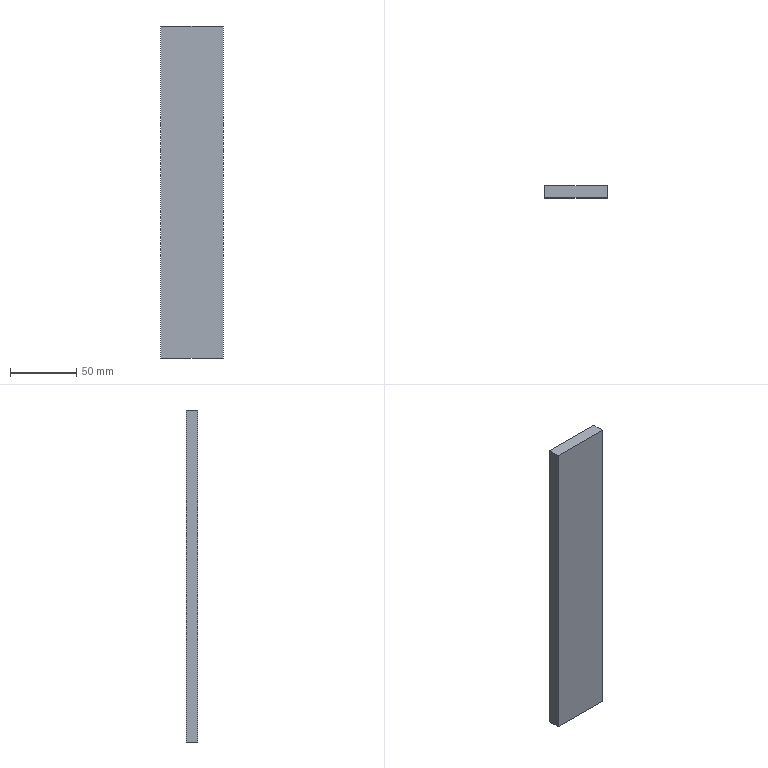Part | STEP file | Squeegee rubber | 1 solid | 6 faces | box 47 x 9 x 250 mm | volume 105750 mm3 | plane 6
STEP:
#1=CARTESIAN_POINT('',(29.,4.5,-250.));
#2=VERTEX_POINT('',#1);
#3=CARTESIAN_POINT('',(29.,-4.5,-250.));
#4=VERTEX_POINT('',#3);
#5=CARTESIAN_POINT('',(29.,4.5,-250.));
#6=DIRECTION('',(0.,-1.,0.));
#7=VECTOR('',#6,1000.);
#8=LINE('',#5,#7);
#9=EDGE_CURVE('',#2,#4,#8,.T.);
#10=ORIENTED_EDGE('',*,*,#9,.F.);
#11=CARTESIAN_POINT('',(76.,4.5,-250.));
#12=VERTEX_POINT('',#11);
#13=CARTESIAN_POINT('',(29.,4.5,-250.));
#14=DIRECTION('',(-1.,0.,0.));
#15=VECTOR('',#14,1000.);
#16=LINE('',#13,#15);
#17=EDGE_CURVE('',#12,#2,#16,.T.);
#18=ORIENTED_EDGE('',*,*,#17,.F.);
#19=CARTESIAN_POINT('',(76.,-4.5,-250.));
#20=VERTEX_POINT('',#19);
#21=CARTESIAN_POINT('',(76.,4.5,-250.));
#22=DIRECTION('',(0.,1.,0.));
#23=VECTOR('',#22,1000.);
#24=LINE('',#21,#23);
#25=EDGE_CURVE('',#20,#12,#24,.T.);
#26=ORIENTED_EDGE('',*,*,#25,.F.);
#27=CARTESIAN_POINT('',(29.,-4.5,-250.));
#28=DIRECTION('',(1.,0.,0.));
#29=VECTOR('',#28,1000.);
#30=LINE('',#27,#29);
#31=EDGE_CURVE('',#4,#20,#30,.T.);
#32=ORIENTED_EDGE('',*,*,#31,.F.);
#33=EDGE_LOOP('',(#10,#18,#26,#32));
#34=FACE_OUTER_BOUND('',#33,.T.);
#35=CARTESIAN_POINT('',(0.,0.,-250.));
#36=DIRECTION('',(0.,0.,-1.));
#37=DIRECTION('',(-1.,0.,0.));
#38=AXIS2_PLACEMENT_3D('',#35,#36,#37);
#39=PLANE('',#38);
#40=ADVANCED_FACE('',(#34),#39,.T.);
#41=CARTESIAN_POINT('',(29.,4.5,0.));
#42=VERTEX_POINT('',#41);
#43=CARTESIAN_POINT('',(29.,-4.5,0.));
#44=VERTEX_POINT('',#43);
#45=CARTESIAN_POINT('',(29.,4.5,0.));
#46=DIRECTION('',(0.,-1.,0.));
#47=VECTOR('',#46,1000.);
#48=LINE('',#45,#47);
#49=EDGE_CURVE('',#42,#44,#48,.T.);
#50=ORIENTED_EDGE('',*,*,#49,.T.);
#51=CARTESIAN_POINT('',(76.,-4.5,0.));
#52=VERTEX_POINT('',#51);
#53=CARTESIAN_POINT('',(29.,-4.5,0.));
#54=DIRECTION('',(1.,0.,0.));
#55=VECTOR('',#54,1000.);
#56=LINE('',#53,#55);
#57=EDGE_CURVE('',#44,#52,#56,.T.);
#58=ORIENTED_EDGE('',*,*,#57,.T.);
#59=CARTESIAN_POINT('',(76.,4.5,0.));
#60=VERTEX_POINT('',#59);
#61=CARTESIAN_POINT('',(76.,4.5,0.));
#62=DIRECTION('',(0.,1.,0.));
#63=VECTOR('',#62,1000.);
#64=LINE('',#61,#63);
#65=EDGE_CURVE('',#52,#60,#64,.T.);
#66=ORIENTED_EDGE('',*,*,#65,.T.);
#67=CARTESIAN_POINT('',(29.,4.5,0.));
#68=DIRECTION('',(-1.,0.,0.));
#69=VECTOR('',#68,1000.);
#70=LINE('',#67,#69);
#71=EDGE_CURVE('',#60,#42,#70,.T.);
#72=ORIENTED_EDGE('',*,*,#71,.T.);
#73=EDGE_LOOP('',(#50,#58,#66,#72));
#74=FACE_OUTER_BOUND('',#73,.T.);
#75=CARTESIAN_POINT('',(0.,0.,0.));
#76=DIRECTION('',(0.,0.,1.));
#77=DIRECTION('',(1.,0.,0.));
#78=AXIS2_PLACEMENT_3D('',#75,#76,#77);
#79=PLANE('',#78);
#80=ADVANCED_FACE('',(#74),#79,.T.);
#81=CARTESIAN_POINT('',(29.,-4.5,-297.854));
#82=DIRECTION('',(0.,0.,1.));
#83=VECTOR('',#82,1000.);
#84=LINE('',#81,#83);
#85=EDGE_CURVE('',#4,#44,#84,.T.);
#86=ORIENTED_EDGE('',*,*,#85,.F.);
#87=ORIENTED_EDGE('',*,*,#31,.T.);
#88=CARTESIAN_POINT('',(76.,-4.5,-297.854));
#89=DIRECTION('',(0.,0.,1.));
#90=VECTOR('',#89,1000.);
#91=LINE('',#88,#90);
#92=EDGE_CURVE('',#20,#52,#91,.T.);
#93=ORIENTED_EDGE('',*,*,#92,.T.);
#94=ORIENTED_EDGE('',*,*,#57,.F.);
#95=EDGE_LOOP('',(#86,#87,#93,#94));
#96=FACE_OUTER_BOUND('',#95,.T.);
#97=CARTESIAN_POINT('',(29.,-4.5,-297.854));
#98=DIRECTION('',(0.,-1.,0.));
#99=DIRECTION('',(0.,0.,-1.));
#100=AXIS2_PLACEMENT_3D('',#97,#98,#99);
#101=PLANE('',#100);
#102=ADVANCED_FACE('',(#96),#101,.T.);
#103=ORIENTED_EDGE('',*,*,#92,.F.);
#104=ORIENTED_EDGE('',*,*,#25,.T.);
#105=CARTESIAN_POINT('',(76.,4.5,-297.854));
#106=DIRECTION('',(0.,0.,1.));
#107=VECTOR('',#106,1000.);
#108=LINE('',#105,#107);
#109=EDGE_CURVE('',#12,#60,#108,.T.);
#110=ORIENTED_EDGE('',*,*,#109,.T.);
#111=ORIENTED_EDGE('',*,*,#65,.F.);
#112=EDGE_LOOP('',(#103,#104,#110,#111));
#113=FACE_OUTER_BOUND('',#112,.T.);
#114=CARTESIAN_POINT('',(76.,4.5,-297.854));
#115=DIRECTION('',(1.,0.,0.));
#116=DIRECTION('',(0.,0.,-1.));
#117=AXIS2_PLACEMENT_3D('',#114,#115,#116);
#118=PLANE('',#117);
#119=ADVANCED_FACE('',(#113),#118,.T.);
#120=ORIENTED_EDGE('',*,*,#109,.F.);
#121=ORIENTED_EDGE('',*,*,#17,.T.);
#122=CARTESIAN_POINT('',(29.,4.5,-297.854));
#123=DIRECTION('',(0.,0.,1.));
#124=VECTOR('',#123,1000.);
#125=LINE('',#122,#124);
#126=EDGE_CURVE('',#2,#42,#125,.T.);
#127=ORIENTED_EDGE('',*,*,#126,.T.);
#128=ORIENTED_EDGE('',*,*,#71,.F.);
#129=EDGE_LOOP('',(#120,#121,#127,#128));
#130=FACE_OUTER_BOUND('',#129,.T.);
#131=CARTESIAN_POINT('',(29.,4.5,-297.854));
#132=DIRECTION('',(0.,1.,0.));
#133=DIRECTION('',(0.,0.,1.));
#134=AXIS2_PLACEMENT_3D('',#131,#132,#133);
#135=PLANE('',#134);
#136=ADVANCED_FACE('',(#130),#135,.T.);
#137=ORIENTED_EDGE('',*,*,#126,.F.);
#138=ORIENTED_EDGE('',*,*,#9,.T.);
#139=ORIENTED_EDGE('',*,*,#85,.T.);
#140=ORIENTED_EDGE('',*,*,#49,.F.);
#141=EDGE_LOOP('',(#137,#138,#139,#140));
#142=FACE_OUTER_BOUND('',#141,.T.);
#143=CARTESIAN_POINT('',(29.,4.5,-297.854));
#144=DIRECTION('',(-1.,0.,0.));
#145=DIRECTION('',(0.,0.,1.));
#146=AXIS2_PLACEMENT_3D('',#143,#144,#145);
#147=PLANE('',#146);
#148=ADVANCED_FACE('',(#142),#147,.T.);
#149=CLOSED_SHELL('',(#40,#80,#102,#119,#136,#148));
#150=MANIFOLD_SOLID_BREP('',#149);
#151=CARTESIAN_POINT('',(0.,0.,0.));
#152=DIRECTION('',(0.,0.,1.));
#153=DIRECTION('',(1.,0.,0.));
#154=AXIS2_PLACEMENT_3D('',#151,#152,#153);
#155=(LENGTH_UNIT()NAMED_UNIT(*)SI_UNIT(.MILLI.,.METRE.));
#156=UNCERTAINTY_MEASURE_WITH_UNIT(LENGTH_MEASURE(0.00001),#155,'','');
#157=(NAMED_UNIT(*)PLANE_ANGLE_UNIT()SI_UNIT($,.RADIAN.));
#158=(NAMED_UNIT(*)SI_UNIT($,.STERADIAN.)SOLID_ANGLE_UNIT());
#159=(GEOMETRIC_REPRESENTATION_CONTEXT(3)GLOBAL_UNCERTAINTY_ASSIGNED_CONTEXT((#156))GLOBAL_UNIT_ASSIGNED_CONTEXT((#155,#157,#158))REPRESENTATION_CONTEXT('',''));
#160=ADVANCED_BREP_SHAPE_REPRESENTATION('',(#150,#154),#159);